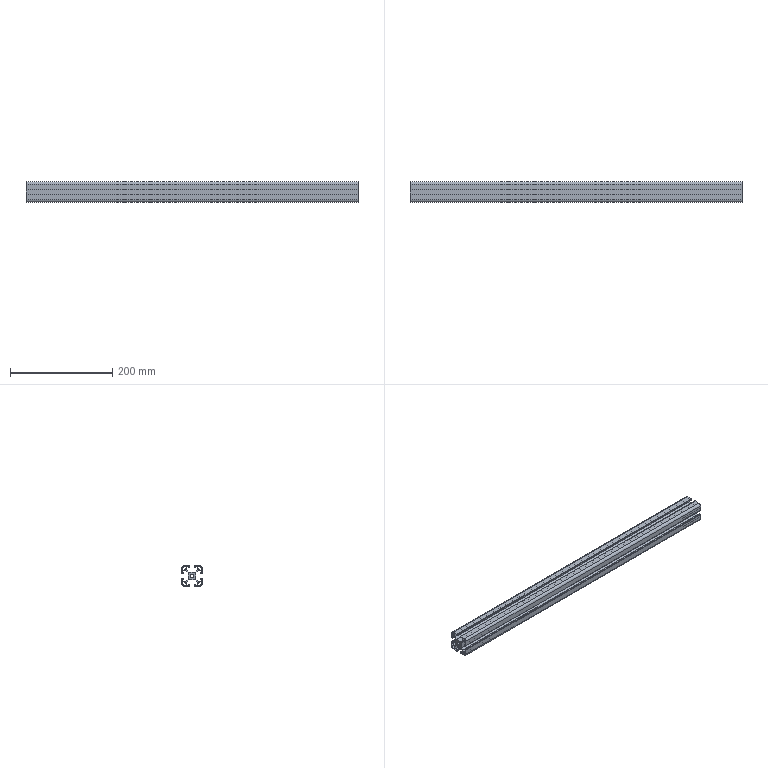Part | SolidWorks | features WeldMemberFeat 1, WeldmentFeature 1 | 1 solid | 104 faces | box 650 x 40 x 40 mm | volume 374755 mm3 | plane 94 | cylinder 10 | commonest cylinder face diameters 5 x4 9 x4 6.8 x2